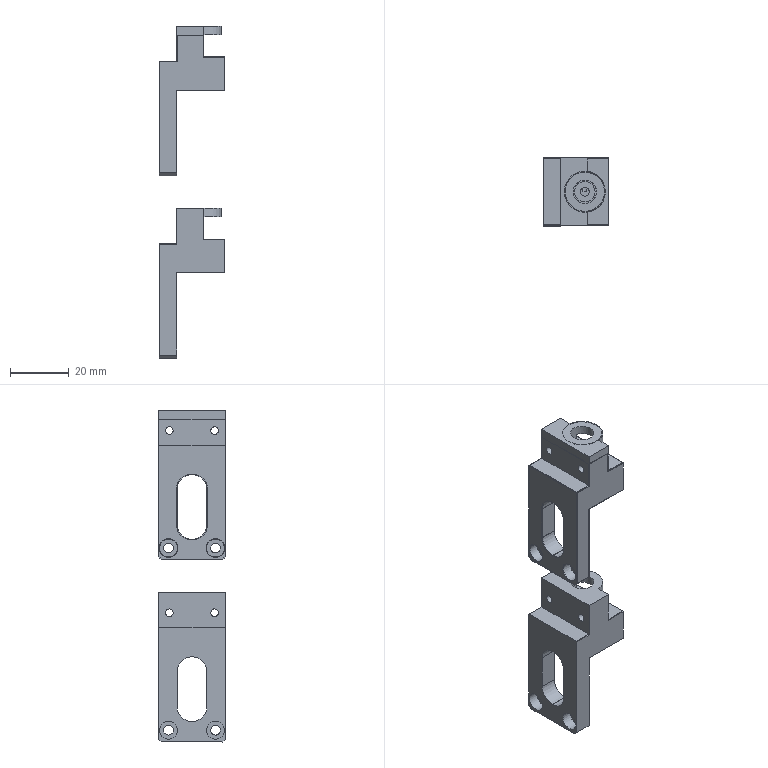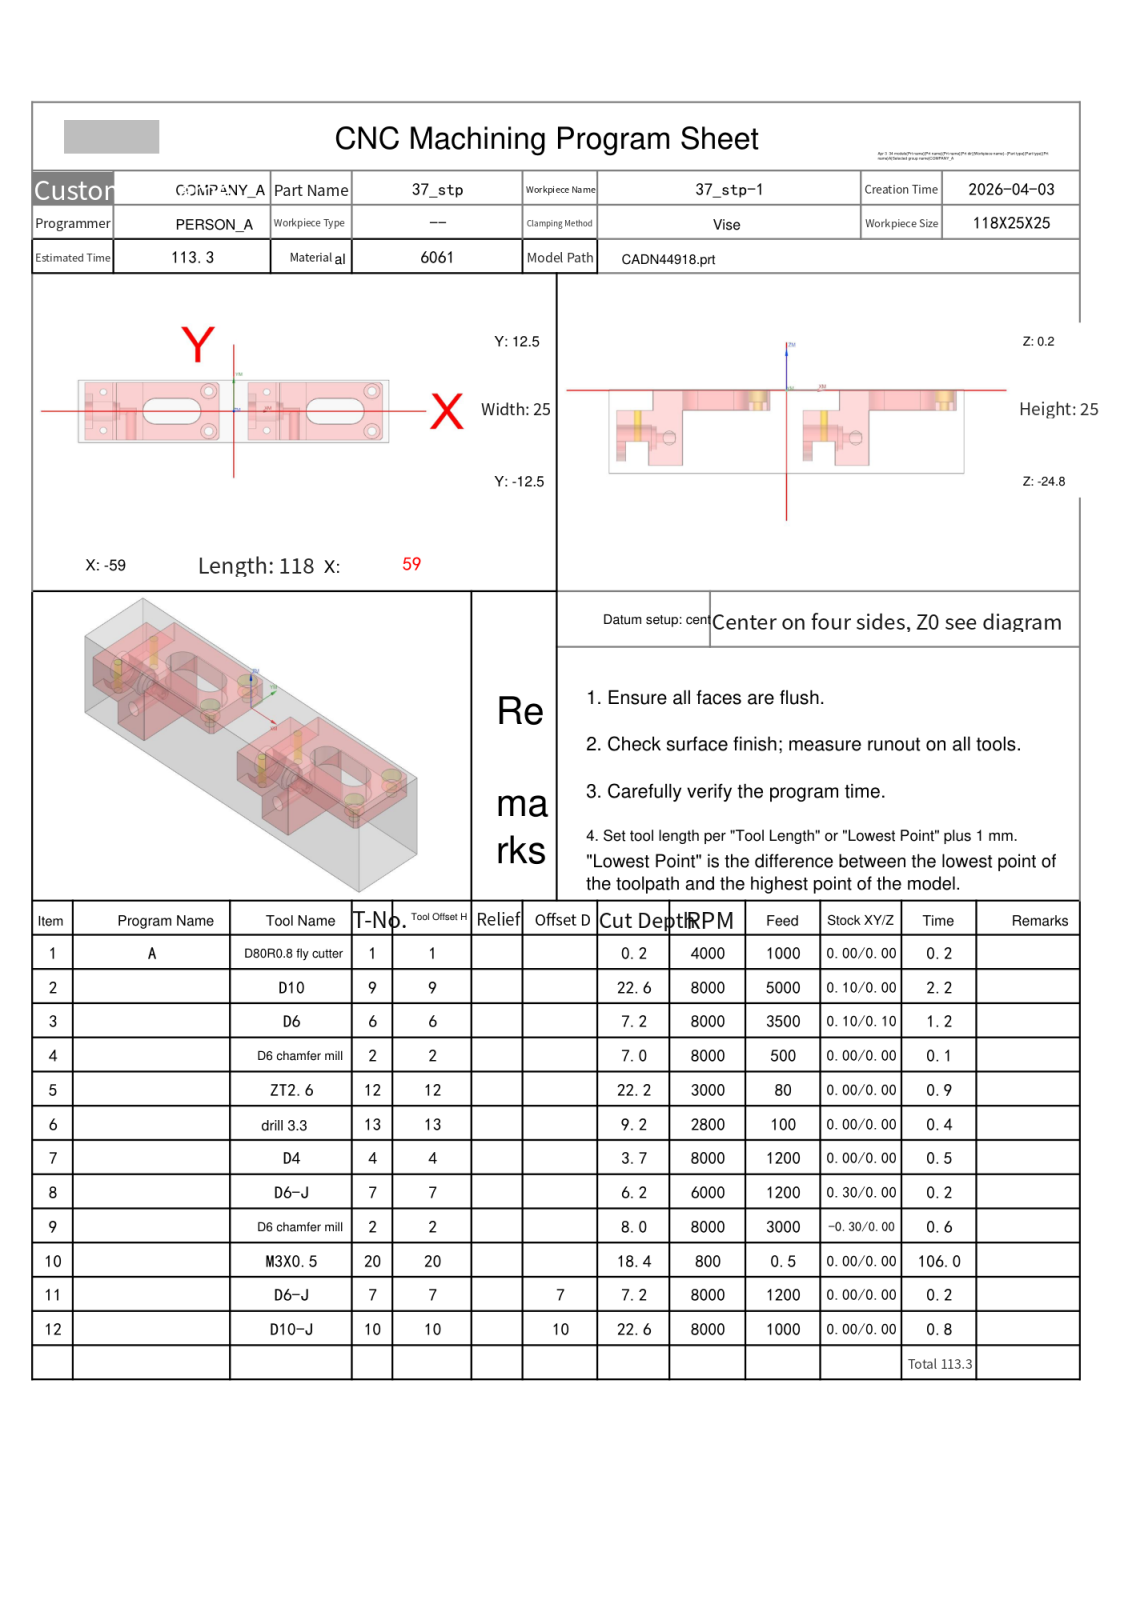NC program | NX | posted by the shop | part box 22.4 x 23 x 113 mm
Lines 2428 to 2531 of 2531:
N12 T10 M06
(D10-J  D=10. R=0. H=10 ce=0.00 di=0.00)
G00 G90 G54 X-57.513 Y17.616 M03 S8000
G43 H10 Z20.
M08
Z-10.7
G01 Z-11.2 F1000.
G41 D10
X-57.497 Y17.417
G03 X-56.5 Y16.5 I.997 J.083
G01 X-45.75
X-6.5
G02 X-2.964 Y15.036 I0.0 J-5.
G01 X-1.964 Y14.036
G02 X-.5 Y10.5 I-3.536 J-3.536
G01 Y-10.5
G02 X-1.964 Y-14.036 I-5. J0.0
G01 X-2.964 Y-15.036
G02 X-6.5 Y-16.5 I-3.536 J3.536
G01 X-56.5
G02 X-61.5 Y-11.5 I0.0 J5.
G01 Y11.5
G02 X-56.5 Y16.5 I5. J0.0
G01 X-56.
G03 X-55. Y17.5 I0.0 J1.
G01 G40 Y17.7
Z-10.7
G00 Z20.
X29.5
Z-10.7
G01 Z-11.2
G41 D10
Y17.5
G03 X30.5 Y16.5 I1. J0.0
G01 X55.5
G02 X59.036 Y15.036 I0.0 J-5.
G01 X60.036 Y14.036
G02 X61.5 Y10.5 I-3.536 J-3.536
G01 Y-10.5
G02 X60.036 Y-14.036 I-5. J0.0
G01 X59.036 Y-15.036
G02 X55.5 Y-16.5 I-3.536 J3.536
G01 X5.5
G02 X.5 Y-11.5 I0.0 J5.
G01 Y11.5
G02 X5.5 Y16.5 I5. J0.0
G01 X30.5
X31.
G03 X32. Y17.5 I0.0 J1.
G01 G40 Y17.7
Z-10.7
G00 Z20.
X4.487 Y17.616
Z-21.9
G01 Z-22.4
G41 D10
X4.503 Y17.417
G03 X5.5 Y16.5 I.997 J.083
G01 X55.5
G02 X59.036 Y15.036 I0.0 J-5.
G01 X60.036 Y14.036
G02 X61.5 Y10.5 I-3.536 J-3.536
G01 Y-10.5
G02 X60.036 Y-14.036 I-5. J0.0
G01 X59.036 Y-15.036
G02 X55.5 Y-16.5 I-3.536 J3.536
G01 X5.5
G02 X.5 Y-11.5 I0.0 J5.
G01 Y11.5
G02 X5.5 Y16.5 I5. J0.0
G01 X6.
G03 X7. Y17.5 I0.0 J1.
G01 G40 Y17.7
X-.616 Y14.318
G41 D10
X-.783 Y14.208
G03 X-1.233 Y13.373 I.55 J-.835
X-1.111 Y12.894 I1. J0.0
G02 X-.5 Y10.5 I-4.389 J-2.394
G01 Y-10.5
G02 X-1.964 Y-14.036 I-5. J0.0
G01 X-2.964 Y-15.036
G02 X-6.5 Y-16.5 I-3.536 J3.536
G01 X-56.5
G02 X-61.5 Y-11.5 I0.0 J5.
G01 Y11.5
G02 X-56.5 Y16.5 I5. J0.0
G01 X-45.75
X-6.5
G02 X-2.964 Y15.036 I0.0 J-5.
G01 X-1.964 Y14.036
G02 X-1.111 Y12.894 I-3.536 J-3.536
X-.893 Y12.444 I-4.389 J-2.394
G03 X.028 Y11.833 I.921 J.389
X.417 Y11.912 I0.0 J1.
G01 G40 X-.212 Y13.336
Z-21.9
G00 Z20.
M05
M09
G91 G28 Z0.0
G91 G28 Y0.0
M30
%